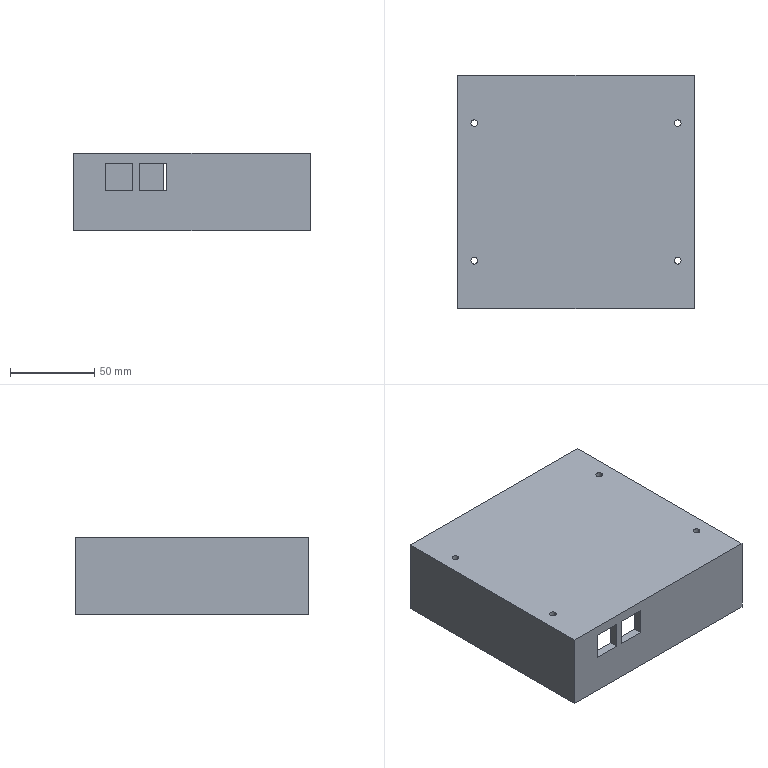Part | SolidWorks | features ICE 9, Extrusion 1, Shell 1 | 1 solid | 35 faces | box 140 x 138 x 46 mm | volume 201014 mm3 | plane 27 | cylinder 8 | commonest cylinder face diameters 4 x8
STEP:
#1=CARTESIAN_POINT('',(-39.512,8.412,41.));
#2=VERTEX_POINT('',#1);
#3=CARTESIAN_POINT('',(-35.512,8.412,41.));
#4=VERTEX_POINT('',#3);
#5=CARTESIAN_POINT('',(-37.512,8.412,41.));
#6=DIRECTION('',(0.,0.,1.));
#7=DIRECTION('',(1.,0.,0.));
#8=AXIS2_PLACEMENT_3D('',#5,#6,#7);
#9=CIRCLE('',#8,2.);
#10=EDGE_CURVE('',#2,#4,#9,.T.);
#11=ORIENTED_EDGE('',*,*,#10,.F.);
#12=CARTESIAN_POINT('',(-39.512,8.412,46.));
#13=VERTEX_POINT('',#12);
#14=CARTESIAN_POINT('',(-39.512,8.412,41.));
#15=DIRECTION('',(0.,0.,1.));
#16=VECTOR('',#15,1000.);
#17=LINE('',#14,#16);
#18=EDGE_CURVE('',#2,#13,#17,.T.);
#19=ORIENTED_EDGE('',*,*,#18,.T.);
#20=CARTESIAN_POINT('',(-35.512,8.412,46.));
#21=VERTEX_POINT('',#20);
#22=CARTESIAN_POINT('',(-37.512,8.412,46.));
#23=DIRECTION('',(0.,0.,1.));
#24=DIRECTION('',(1.,0.,0.));
#25=AXIS2_PLACEMENT_3D('',#22,#23,#24);
#26=CIRCLE('',#25,2.);
#27=EDGE_CURVE('',#13,#21,#26,.T.);
#28=ORIENTED_EDGE('',*,*,#27,.T.);
#29=CARTESIAN_POINT('',(-35.512,8.412,41.));
#30=DIRECTION('',(0.,0.,1.));
#31=VECTOR('',#30,1000.);
#32=LINE('',#29,#31);
#33=EDGE_CURVE('',#4,#21,#32,.T.);
#34=ORIENTED_EDGE('',*,*,#33,.F.);
#35=EDGE_LOOP('',(#11,#19,#28,#34));
#36=FACE_OUTER_BOUND('',#35,.T.);
#37=CARTESIAN_POINT('',(-37.512,8.412,41.));
#38=DIRECTION('',(0.,0.,1.));
#39=DIRECTION('',(1.,0.,0.));
#40=AXIS2_PLACEMENT_3D('',#37,#38,#39);
#41=CYLINDRICAL_SURFACE('',#40,2.);
#42=ADVANCED_FACE('',(#36),#41,.F.);
#43=CARTESIAN_POINT('',(80.888,89.812,41.));
#44=VERTEX_POINT('',#43);
#45=CARTESIAN_POINT('',(84.888,89.812,41.));
#46=VERTEX_POINT('',#45);
#47=CARTESIAN_POINT('',(82.888,89.812,41.));
#48=DIRECTION('',(0.,0.,1.));
#49=DIRECTION('',(1.,0.,0.));
#50=AXIS2_PLACEMENT_3D('',#47,#48,#49);
#51=CIRCLE('',#50,2.);
#52=EDGE_CURVE('',#44,#46,#51,.T.);
#53=ORIENTED_EDGE('',*,*,#52,.F.);
#54=CARTESIAN_POINT('',(80.888,89.812,46.));
#55=VERTEX_POINT('',#54);
#56=CARTESIAN_POINT('',(80.888,89.812,41.));
#57=DIRECTION('',(0.,0.,1.));
#58=VECTOR('',#57,1000.);
#59=LINE('',#56,#58);
#60=EDGE_CURVE('',#44,#55,#59,.T.);
#61=ORIENTED_EDGE('',*,*,#60,.T.);
#62=CARTESIAN_POINT('',(84.888,89.812,46.));
#63=VERTEX_POINT('',#62);
#64=CARTESIAN_POINT('',(82.888,89.812,46.));
#65=DIRECTION('',(0.,0.,1.));
#66=DIRECTION('',(1.,0.,0.));
#67=AXIS2_PLACEMENT_3D('',#64,#65,#66);
#68=CIRCLE('',#67,2.);
#69=EDGE_CURVE('',#55,#63,#68,.T.);
#70=ORIENTED_EDGE('',*,*,#69,.T.);
#71=CARTESIAN_POINT('',(84.888,89.812,41.));
#72=DIRECTION('',(0.,0.,1.));
#73=VECTOR('',#72,1000.);
#74=LINE('',#71,#73);
#75=EDGE_CURVE('',#46,#63,#74,.T.);
#76=ORIENTED_EDGE('',*,*,#75,.F.);
#77=EDGE_LOOP('',(#53,#61,#70,#76));
#78=FACE_OUTER_BOUND('',#77,.T.);
#79=CARTESIAN_POINT('',(82.888,89.812,41.));
#80=DIRECTION('',(0.,0.,1.));
#81=DIRECTION('',(1.,0.,0.));
#82=AXIS2_PLACEMENT_3D('',#79,#80,#81);
#83=CYLINDRICAL_SURFACE('',#82,2.);
#84=ADVANCED_FACE('',(#78),#83,.F.);
#85=CARTESIAN_POINT('',(80.888,8.412,41.));
#86=VERTEX_POINT('',#85);
#87=CARTESIAN_POINT('',(84.888,8.412,41.));
#88=VERTEX_POINT('',#87);
#89=CARTESIAN_POINT('',(82.888,8.412,41.));
#90=DIRECTION('',(0.,0.,1.));
#91=DIRECTION('',(1.,0.,0.));
#92=AXIS2_PLACEMENT_3D('',#89,#90,#91);
#93=CIRCLE('',#92,2.);
#94=EDGE_CURVE('',#86,#88,#93,.T.);
#95=ORIENTED_EDGE('',*,*,#94,.F.);
#96=CARTESIAN_POINT('',(80.888,8.412,46.));
#97=VERTEX_POINT('',#96);
#98=CARTESIAN_POINT('',(80.888,8.412,41.));
#99=DIRECTION('',(0.,0.,1.));
#100=VECTOR('',#99,1000.);
#101=LINE('',#98,#100);
#102=EDGE_CURVE('',#86,#97,#101,.T.);
#103=ORIENTED_EDGE('',*,*,#102,.T.);
#104=CARTESIAN_POINT('',(84.888,8.412,46.));
#105=VERTEX_POINT('',#104);
#106=CARTESIAN_POINT('',(82.888,8.412,46.));
#107=DIRECTION('',(0.,0.,1.));
#108=DIRECTION('',(1.,0.,0.));
#109=AXIS2_PLACEMENT_3D('',#106,#107,#108);
#110=CIRCLE('',#109,2.);
#111=EDGE_CURVE('',#97,#105,#110,.T.);
#112=ORIENTED_EDGE('',*,*,#111,.T.);
#113=CARTESIAN_POINT('',(84.888,8.412,41.));
#114=DIRECTION('',(0.,0.,1.));
#115=VECTOR('',#114,1000.);
#116=LINE('',#113,#115);
#117=EDGE_CURVE('',#88,#105,#116,.T.);
#118=ORIENTED_EDGE('',*,*,#117,.F.);
#119=EDGE_LOOP('',(#95,#103,#112,#118));
#120=FACE_OUTER_BOUND('',#119,.T.);
#121=CARTESIAN_POINT('',(82.888,8.412,41.));
#122=DIRECTION('',(0.,0.,1.));
#123=DIRECTION('',(1.,0.,0.));
#124=AXIS2_PLACEMENT_3D('',#121,#122,#123);
#125=CYLINDRICAL_SURFACE('',#124,2.);
#126=ADVANCED_FACE('',(#120),#125,.F.);
#127=CARTESIAN_POINT('',(-39.512,89.812,41.));
#128=VERTEX_POINT('',#127);
#129=CARTESIAN_POINT('',(-35.512,89.812,41.));
#130=VERTEX_POINT('',#129);
#131=CARTESIAN_POINT('',(-37.512,89.812,41.));
#132=DIRECTION('',(0.,0.,1.));
#133=DIRECTION('',(1.,0.,0.));
#134=AXIS2_PLACEMENT_3D('',#131,#132,#133);
#135=CIRCLE('',#134,2.);
#136=EDGE_CURVE('',#128,#130,#135,.T.);
#137=ORIENTED_EDGE('',*,*,#136,.F.);
#138=CARTESIAN_POINT('',(-39.512,89.812,46.));
#139=VERTEX_POINT('',#138);
#140=CARTESIAN_POINT('',(-39.512,89.812,41.));
#141=DIRECTION('',(0.,0.,1.));
#142=VECTOR('',#141,1000.);
#143=LINE('',#140,#142);
#144=EDGE_CURVE('',#128,#139,#143,.T.);
#145=ORIENTED_EDGE('',*,*,#144,.T.);
#146=CARTESIAN_POINT('',(-35.512,89.812,46.));
#147=VERTEX_POINT('',#146);
#148=CARTESIAN_POINT('',(-37.512,89.812,46.));
#149=DIRECTION('',(0.,0.,1.));
#150=DIRECTION('',(1.,0.,0.));
#151=AXIS2_PLACEMENT_3D('',#148,#149,#150);
#152=CIRCLE('',#151,2.);
#153=EDGE_CURVE('',#139,#147,#152,.T.);
#154=ORIENTED_EDGE('',*,*,#153,.T.);
#155=CARTESIAN_POINT('',(-35.512,89.812,41.));
#156=DIRECTION('',(0.,0.,1.));
#157=VECTOR('',#156,1000.);
#158=LINE('',#155,#157);
#159=EDGE_CURVE('',#130,#147,#158,.T.);
#160=ORIENTED_EDGE('',*,*,#159,.F.);
#161=EDGE_LOOP('',(#137,#145,#154,#160));
#162=FACE_OUTER_BOUND('',#161,.T.);
#163=CARTESIAN_POINT('',(-37.512,89.812,41.));
#164=DIRECTION('',(0.,0.,1.));
#165=DIRECTION('',(1.,0.,0.));
#166=AXIS2_PLACEMENT_3D('',#163,#164,#165);
#167=CYLINDRICAL_SURFACE('',#166,2.);
#168=ADVANCED_FACE('',(#162),#167,.F.);
#169=CARTESIAN_POINT('',(-47.312,118.112,0.));
#170=VERTEX_POINT('',#169);
#171=CARTESIAN_POINT('',(-47.312,-19.888,0.));
#172=VERTEX_POINT('',#171);
#173=CARTESIAN_POINT('',(-47.312,118.112,0.));
#174=DIRECTION('',(0.,-1.,0.));
#175=VECTOR('',#174,1000.);
#176=LINE('',#173,#175);
#177=EDGE_CURVE('',#170,#172,#176,.T.);
#178=ORIENTED_EDGE('',*,*,#177,.T.);
#179=CARTESIAN_POINT('',(-47.312,-19.888,46.));
#180=VERTEX_POINT('',#179);
#181=CARTESIAN_POINT('',(-47.312,-19.888,46.));
#182=DIRECTION('',(0.,0.,-1.));
#183=VECTOR('',#182,1000.);
#184=LINE('',#181,#183);
#185=EDGE_CURVE('',#180,#172,#184,.T.);
#186=ORIENTED_EDGE('',*,*,#185,.F.);
#187=CARTESIAN_POINT('',(-47.312,118.112,46.));
#188=VERTEX_POINT('',#187);
#189=CARTESIAN_POINT('',(-47.312,118.112,46.));
#190=DIRECTION('',(0.,-1.,0.));
#191=VECTOR('',#190,1000.);
#192=LINE('',#189,#191);
#193=EDGE_CURVE('',#188,#180,#192,.T.);
#194=ORIENTED_EDGE('',*,*,#193,.F.);
#195=CARTESIAN_POINT('',(-47.312,118.112,46.));
#196=DIRECTION('',(0.,0.,-1.));
#197=VECTOR('',#196,1000.);
#198=LINE('',#195,#197);
#199=EDGE_CURVE('',#188,#170,#198,.T.);
#200=ORIENTED_EDGE('',*,*,#199,.T.);
#201=EDGE_LOOP('',(#178,#186,#194,#200));
#202=FACE_OUTER_BOUND('',#201,.T.);
#203=CARTESIAN_POINT('',(-47.312,118.112,46.));
#204=DIRECTION('',(1.,0.,0.));
#205=DIRECTION('',(0.,1.,0.));
#206=AXIS2_PLACEMENT_3D('',#203,#204,#205);
#207=PLANE('',#206);
#208=ADVANCED_FACE('',(#202),#207,.F.);
#209=CARTESIAN_POINT('',(-8.312,-19.888,24.));
#210=VERTEX_POINT('',#209);
#211=CARTESIAN_POINT('',(7.688,-19.888,24.));
#212=VERTEX_POINT('',#211);
#213=CARTESIAN_POINT('',(-8.312,-19.888,24.));
#214=DIRECTION('',(1.,0.,0.));
#215=VECTOR('',#214,1000.);
#216=LINE('',#213,#215);
#217=EDGE_CURVE('',#210,#212,#216,.T.);
#218=ORIENTED_EDGE('',*,*,#217,.F.);
#219=CARTESIAN_POINT('',(-8.312,-19.888,40.));
#220=VERTEX_POINT('',#219);
#221=CARTESIAN_POINT('',(-8.312,-19.888,40.));
#222=DIRECTION('',(0.,0.,-1.));
#223=VECTOR('',#222,1000.);
#224=LINE('',#221,#223);
#225=EDGE_CURVE('',#220,#210,#224,.T.);
#226=ORIENTED_EDGE('',*,*,#225,.F.);
#227=CARTESIAN_POINT('',(7.688,-19.888,40.));
#228=VERTEX_POINT('',#227);
#229=CARTESIAN_POINT('',(-8.312,-19.888,40.));
#230=DIRECTION('',(-1.,0.,0.));
#231=VECTOR('',#230,1000.);
#232=LINE('',#229,#231);
#233=EDGE_CURVE('',#228,#220,#232,.T.);
#234=ORIENTED_EDGE('',*,*,#233,.F.);
#235=CARTESIAN_POINT('',(7.688,-19.888,40.));
#236=DIRECTION('',(0.,0.,1.));
#237=VECTOR('',#236,1000.);
#238=LINE('',#235,#237);
#239=EDGE_CURVE('',#212,#228,#238,.T.);
#240=ORIENTED_EDGE('',*,*,#239,.F.);
#241=EDGE_LOOP('',(#218,#226,#234,#240));
#242=FACE_BOUND('',#241,.T.);
#243=CARTESIAN_POINT('',(-28.312,-19.888,24.));
#244=VERTEX_POINT('',#243);
#245=CARTESIAN_POINT('',(-12.312,-19.888,24.));
#246=VERTEX_POINT('',#245);
#247=CARTESIAN_POINT('',(-28.312,-19.888,24.));
#248=DIRECTION('',(1.,0.,0.));
#249=VECTOR('',#248,1000.);
#250=LINE('',#247,#249);
#251=EDGE_CURVE('',#244,#246,#250,.T.);
#252=ORIENTED_EDGE('',*,*,#251,.F.);
#253=CARTESIAN_POINT('',(-28.312,-19.888,40.));
#254=VERTEX_POINT('',#253);
#255=CARTESIAN_POINT('',(-28.312,-19.888,40.));
#256=DIRECTION('',(0.,0.,-1.));
#257=VECTOR('',#256,1000.);
#258=LINE('',#255,#257);
#259=EDGE_CURVE('',#254,#244,#258,.T.);
#260=ORIENTED_EDGE('',*,*,#259,.F.);
#261=CARTESIAN_POINT('',(-12.312,-19.888,40.));
#262=VERTEX_POINT('',#261);
#263=CARTESIAN_POINT('',(-28.312,-19.888,40.));
#264=DIRECTION('',(-1.,0.,0.));
#265=VECTOR('',#264,1000.);
#266=LINE('',#263,#265);
#267=EDGE_CURVE('',#262,#254,#266,.T.);
#268=ORIENTED_EDGE('',*,*,#267,.F.);
#269=CARTESIAN_POINT('',(-12.312,-19.888,40.));
#270=DIRECTION('',(0.,0.,1.));
#271=VECTOR('',#270,1000.);
#272=LINE('',#269,#271);
#273=EDGE_CURVE('',#246,#262,#272,.T.);
#274=ORIENTED_EDGE('',*,*,#273,.F.);
#275=EDGE_LOOP('',(#252,#260,#268,#274));
#276=FACE_BOUND('',#275,.T.);
#277=CARTESIAN_POINT('',(92.688,-19.888,0.));
#278=VERTEX_POINT('',#277);
#279=CARTESIAN_POINT('',(-47.312,-19.888,0.));
#280=DIRECTION('',(1.,0.,0.));
#281=VECTOR('',#280,1000.);
#282=LINE('',#279,#281);
#283=EDGE_CURVE('',#172,#278,#282,.T.);
#284=ORIENTED_EDGE('',*,*,#283,.T.);
#285=CARTESIAN_POINT('',(92.688,-19.888,46.));
#286=VERTEX_POINT('',#285);
#287=CARTESIAN_POINT('',(92.688,-19.888,46.));
#288=DIRECTION('',(0.,0.,-1.));
#289=VECTOR('',#288,1000.);
#290=LINE('',#287,#289);
#291=EDGE_CURVE('',#286,#278,#290,.T.);
#292=ORIENTED_EDGE('',*,*,#291,.F.);
#293=CARTESIAN_POINT('',(-47.312,-19.888,46.));
#294=DIRECTION('',(1.,0.,0.));
#295=VECTOR('',#294,1000.);
#296=LINE('',#293,#295);
#297=EDGE_CURVE('',#180,#286,#296,.T.);
#298=ORIENTED_EDGE('',*,*,#297,.F.);
#299=ORIENTED_EDGE('',*,*,#185,.T.);
#300=EDGE_LOOP('',(#284,#292,#298,#299));
#301=FACE_OUTER_BOUND('',#300,.T.);
#302=CARTESIAN_POINT('',(-47.312,-19.888,46.));
#303=DIRECTION('',(0.,1.,0.));
#304=DIRECTION('',(0.,0.,1.));
#305=AXIS2_PLACEMENT_3D('',#302,#303,#304);
#306=PLANE('',#305);
#307=ADVANCED_FACE('',(#242,#276,#301),#306,.F.);
#308=CARTESIAN_POINT('',(92.688,118.112,0.));
#309=VERTEX_POINT('',#308);
#310=CARTESIAN_POINT('',(92.688,118.112,0.));
#311=DIRECTION('',(0.,1.,0.));
#312=VECTOR('',#311,1000.);
#313=LINE('',#310,#312);
#314=EDGE_CURVE('',#278,#309,#313,.T.);
#315=ORIENTED_EDGE('',*,*,#314,.T.);
#316=CARTESIAN_POINT('',(92.688,118.112,46.));
#317=VERTEX_POINT('',#316);
#318=CARTESIAN_POINT('',(92.688,118.112,46.));
#319=DIRECTION('',(0.,0.,-1.));
#320=VECTOR('',#319,1000.);
#321=LINE('',#318,#320);
#322=EDGE_CURVE('',#317,#309,#321,.T.);
#323=ORIENTED_EDGE('',*,*,#322,.F.);
#324=CARTESIAN_POINT('',(92.688,118.112,46.));
#325=DIRECTION('',(0.,1.,0.));
#326=VECTOR('',#325,1000.);
#327=LINE('',#324,#326);
#328=EDGE_CURVE('',#286,#317,#327,.T.);
#329=ORIENTED_EDGE('',*,*,#328,.F.);
#330=ORIENTED_EDGE('',*,*,#291,.T.);
#331=EDGE_LOOP('',(#315,#323,#329,#330));
#332=FACE_OUTER_BOUND('',#331,.T.);
#333=CARTESIAN_POINT('',(92.688,118.112,46.));
#334=DIRECTION('',(-1.,0.,0.));
#335=DIRECTION('',(0.,-1.,0.));
#336=AXIS2_PLACEMENT_3D('',#333,#334,#335);
#337=PLANE('',#336);
#338=ADVANCED_FACE('',(#332),#337,.F.);
#339=CARTESIAN_POINT('',(76.688,118.112,40.));
#340=VERTEX_POINT('',#339);
#341=CARTESIAN_POINT('',(76.688,118.112,25.));
#342=VERTEX_POINT('',#341);
#343=CARTESIAN_POINT('',(76.688,118.112,0.));
#344=DIRECTION('',(0.,0.,-1.));
#345=VECTOR('',#344,1000.);
#346=LINE('',#343,#345);
#347=EDGE_CURVE('',#340,#342,#346,.T.);
#348=ORIENTED_EDGE('',*,*,#347,.F.);
#349=CARTESIAN_POINT('',(61.688,118.112,40.));
#350=VERTEX_POINT('',#349);
#351=CARTESIAN_POINT('',(0.,118.112,40.));
#352=DIRECTION('',(1.,0.,0.));
#353=VECTOR('',#352,1000.);
#354=LINE('',#351,#353);
#355=EDGE_CURVE('',#350,#340,#354,.T.);
#356=ORIENTED_EDGE('',*,*,#355,.F.);
#357=CARTESIAN_POINT('',(61.688,118.112,25.));
#358=VERTEX_POINT('',#357);
#359=CARTESIAN_POINT('',(61.688,118.112,0.));
#360=DIRECTION('',(0.,0.,-1.));
#361=VECTOR('',#360,1000.);
#362=LINE('',#359,#361);
#363=EDGE_CURVE('',#350,#358,#362,.T.);
#364=ORIENTED_EDGE('',*,*,#363,.T.);
#365=CARTESIAN_POINT('',(0.,118.112,25.));
#366=DIRECTION('',(1.,0.,0.));
#367=VECTOR('',#366,1000.);
#368=LINE('',#365,#367);
#369=EDGE_CURVE('',#358,#342,#368,.T.);
#370=ORIENTED_EDGE('',*,*,#369,.T.);
#371=EDGE_LOOP('',(#348,#356,#364,#370));
#372=FACE_BOUND('',#371,.T.);
#373=CARTESIAN_POINT('',(22.688,118.112,40.));
#374=VERTEX_POINT('',#373);
#375=CARTESIAN_POINT('',(22.688,118.112,22.));
#376=VERTEX_POINT('',#375);
#377=CARTESIAN_POINT('',(22.688,118.112,0.));
#378=DIRECTION('',(0.,0.,-1.));
#379=VECTOR('',#378,1000.);
#380=LINE('',#377,#379);
#381=EDGE_CURVE('',#374,#376,#380,.T.);
#382=ORIENTED_EDGE('',*,*,#381,.F.);
#383=CARTESIAN_POINT('',(5.688,118.112,40.));
#384=VERTEX_POINT('',#383);
#385=CARTESIAN_POINT('',(0.,118.112,40.));
#386=DIRECTION('',(1.,0.,0.));
#387=VECTOR('',#386,1000.);
#388=LINE('',#385,#387);
#389=EDGE_CURVE('',#384,#374,#388,.T.);
#390=ORIENTED_EDGE('',*,*,#389,.F.);
#391=CARTESIAN_POINT('',(5.688,118.112,22.));
#392=VERTEX_POINT('',#391);
#393=CARTESIAN_POINT('',(5.688,118.112,0.));
#394=DIRECTION('',(0.,0.,-1.));
#395=VECTOR('',#394,1000.);
#396=LINE('',#393,#395);
#397=EDGE_CURVE('',#384,#392,#396,.T.);
#398=ORIENTED_EDGE('',*,*,#397,.T.);
#399=CARTESIAN_POINT('',(0.,118.112,22.));
#400=DIRECTION('',(1.,0.,0.));
#401=VECTOR('',#400,1000.);
#402=LINE('',#399,#401);
#403=EDGE_CURVE('',#392,#376,#402,.T.);
#404=ORIENTED_EDGE('',*,*,#403,.T.);
#405=EDGE_LOOP('',(#382,#390,#398,#404));
#406=FACE_BOUND('',#405,.T.);
#407=CARTESIAN_POINT('',(-47.312,118.112,0.));
#408=DIRECTION('',(-1.,0.,0.));
#409=VECTOR('',#408,1000.);
#410=LINE('',#407,#409);
#411=EDGE_CURVE('',#309,#170,#410,.T.);
#412=ORIENTED_EDGE('',*,*,#411,.T.);
#413=ORIENTED_EDGE('',*,*,#199,.F.);
#414=CARTESIAN_POINT('',(-47.312,118.112,46.));
#415=DIRECTION('',(-1.,0.,0.));
#416=VECTOR('',#415,1000.);
#417=LINE('',#414,#416);
#418=EDGE_CURVE('',#317,#188,#417,.T.);
#419=ORIENTED_EDGE('',*,*,#418,.F.);
#420=ORIENTED_EDGE('',*,*,#322,.T.);
#421=EDGE_LOOP('',(#412,#413,#419,#420));
#422=FACE_OUTER_BOUND('',#421,.T.);
#423=CARTESIAN_POINT('',(-47.312,118.112,46.));
#424=DIRECTION('',(0.,-1.,0.));
#425=DIRECTION('',(0.,0.,-1.));
#426=AXIS2_PLACEMENT_3D('',#423,#424,#425);
#427=PLANE('',#426);
#428=ADVANCED_FACE('',(#372,#406,#422),#427,.F.);
#429=CARTESIAN_POINT('',(-37.512,8.412,46.));
#430=DIRECTION('',(0.,0.,1.));
#431=DIRECTION('',(1.,0.,0.));
#432=AXIS2_PLACEMENT_3D('',#429,#430,#431);
#433=CIRCLE('',#432,2.);
#434=EDGE_CURVE('',#21,#13,#433,.T.);
#435=ORIENTED_EDGE('',*,*,#434,.F.);
#436=ORIENTED_EDGE('',*,*,#27,.F.);
#437=EDGE_LOOP('',(#435,#436));
#438=FACE_BOUND('',#437,.T.);
#439=CARTESIAN_POINT('',(82.888,89.812,46.));
#440=DIRECTION('',(0.,0.,1.));
#441=DIRECTION('',(1.,0.,0.));
#442=AXIS2_PLACEMENT_3D('',#439,#440,#441);
#443=CIRCLE('',#442,2.);
#444=EDGE_CURVE('',#63,#55,#443,.T.);
#445=ORIENTED_EDGE('',*,*,#444,.F.);
#446=ORIENTED_EDGE('',*,*,#69,.F.);
#447=EDGE_LOOP('',(#445,#446));
#448=FACE_BOUND('',#447,.T.);
#449=CARTESIAN_POINT('',(82.888,8.412,46.));
#450=DIRECTION('',(0.,0.,1.));
#451=DIRECTION('',(1.,0.,0.));
#452=AXIS2_PLACEMENT_3D('',#449,#450,#451);
#453=CIRCLE('',#452,2.);
#454=EDGE_CURVE('',#105,#97,#453,.T.);
#455=ORIENTED_EDGE('',*,*,#454,.F.);
#456=ORIENTED_EDGE('',*,*,#111,.F.);
#457=EDGE_LOOP('',(#455,#456));
#458=FACE_BOUND('',#457,.T.);
#459=CARTESIAN_POINT('',(-37.512,89.812,46.));
#460=DIRECTION('',(0.,0.,1.));
#461=DIRECTION('',(1.,0.,0.));
#462=AXIS2_PLACEMENT_3D('',#459,#460,#461);
#463=CIRCLE('',#462,2.);
#464=EDGE_CURVE('',#147,#139,#463,.T.);
#465=ORIENTED_EDGE('',*,*,#464,.F.);
#466=ORIENTED_EDGE('',*,*,#153,.F.);
#467=EDGE_LOOP('',(#465,#466));
#468=FACE_BOUND('',#467,.T.);
#469=ORIENTED_EDGE('',*,*,#193,.T.);
#470=ORIENTED_EDGE('',*,*,#297,.T.);
#471=ORIENTED_EDGE('',*,*,#328,.T.);
#472=ORIENTED_EDGE('',*,*,#418,.T.);
#473=EDGE_LOOP('',(#469,#470,#471,#472));
#474=FACE_OUTER_BOUND('',#473,.T.);
#475=CARTESIAN_POINT('',(0.,0.,46.));
#476=DIRECTION('',(0.,0.,1.));
#477=DIRECTION('',(1.,0.,0.));
#478=AXIS2_PLACEMENT_3D('',#475,#476,#477);
#479=PLANE('',#478);
#480=ADVANCED_FACE('',(#438,#448,#458,#468,#474),#479,.T.);
#481=CARTESIAN_POINT('',(87.688,113.112,0.));
#482=VERTEX_POINT('',#481);
#483=CARTESIAN_POINT('',(-42.312,113.112,0.));
#484=VERTEX_POINT('',#483);
#485=CARTESIAN_POINT('',(-47.312,113.112,0.));
#486=DIRECTION('',(-1.,0.,0.));
#487=VECTOR('',#486,1000.);
#488=LINE('',#485,#487);
#489=EDGE_CURVE('',#482,#484,#488,.T.);
#490=ORIENTED_EDGE('',*,*,#489,.T.);
#491=CARTESIAN_POINT('',(-42.312,-14.888,0.));
#492=VERTEX_POINT('',#491);
#493=CARTESIAN_POINT('',(-42.312,118.112,0.));
#494=DIRECTION('',(0.,-1.,0.));
#495=VECTOR('',#494,1000.);
#496=LINE('',#493,#495);
#497=EDGE_CURVE('',#484,#492,#496,.T.);
#498=ORIENTED_EDGE('',*,*,#497,.T.);
#499=CARTESIAN_POINT('',(87.688,-14.888,0.));
#500=VERTEX_POINT('',#499);
#501=CARTESIAN_POINT('',(-47.312,-14.888,0.));
#502=DIRECTION('',(1.,0.,0.));
#503=VECTOR('',#502,1000.);
#504=LINE('',#501,#503);
#505=EDGE_CURVE('',#492,#500,#504,.T.);
#506=ORIENTED_EDGE('',*,*,#505,.T.);
#507=CARTESIAN_POINT('',(87.688,118.112,0.));
#508=DIRECTION('',(0.,1.,0.));
#509=VECTOR('',#508,1000.);
#510=LINE('',#507,#509);
#511=EDGE_CURVE('',#500,#482,#510,.T.);
#512=ORIENTED_EDGE('',*,*,#511,.T.);
#513=EDGE_LOOP('',(#490,#498,#506,#512));
#514=FACE_BOUND('',#513,.T.);
#515=ORIENTED_EDGE('',*,*,#177,.F.);
#516=ORIENTED_EDGE('',*,*,#411,.F.);
#517=ORIENTED_EDGE('',*,*,#314,.F.);
#518=ORIENTED_EDGE('',*,*,#283,.F.);
#519=EDGE_LOOP('',(#515,#516,#517,#518));
#520=FACE_OUTER_BOUND('',#519,.T.);
#521=CARTESIAN_POINT('',(0.,0.,0.));
#522=DIRECTION('',(0.,0.,1.));
#523=DIRECTION('',(1.,0.,0.));
#524=AXIS2_PLACEMENT_3D('',#521,#522,#523);
#525=PLANE('',#524);
#526=ADVANCED_FACE('',(#514,#520),#525,.F.);
#527=ORIENTED_EDGE('',*,*,#497,.F.);
#528=CARTESIAN_POINT('',(-42.312,113.112,41.));
#529=VERTEX_POINT('',#528);
#530=CARTESIAN_POINT('',(-42.312,113.112,46.));
#531=DIRECTION('',(0.,0.,-1.));
#532=VECTOR('',#531,1000.);
#533=LINE('',#530,#532);
#534=EDGE_CURVE('',#529,#484,#533,.T.);
#535=ORIENTED_EDGE('',*,*,#534,.F.);
#536=CARTESIAN_POINT('',(-42.312,-14.888,41.));
#537=VERTEX_POINT('',#536);
#538=CARTESIAN_POINT('',(-42.312,118.112,41.));
#539=DIRECTION('',(0.,-1.,0.));
#540=VECTOR('',#539,1000.);
#541=LINE('',#538,#540);
#542=EDGE_CURVE('',#529,#537,#541,.T.);
#543=ORIENTED_EDGE('',*,*,#542,.T.);
#544=CARTESIAN_POINT('',(-42.312,-14.888,46.));
#545=DIRECTION('',(0.,0.,-1.));
#546=VECTOR('',#545,1000.);
#547=LINE('',#544,#546);
#548=EDGE_CURVE('',#537,#492,#547,.T.);
#549=ORIENTED_EDGE('',*,*,#548,.T.);
#550=EDGE_LOOP('',(#527,#535,#543,#549));
#551=FACE_OUTER_BOUND('',#550,.T.);
#552=CARTESIAN_POINT('',(-42.312,118.112,46.));
#553=DIRECTION('',(1.,0.,0.));
#554=DIRECTION('',(0.,1.,0.));
#555=AXIS2_PLACEMENT_3D('',#552,#553,#554);
#556=PLANE('',#555);
#557=ADVANCED_FACE('',(#551),#556,.T.);
#558=CARTESIAN_POINT('',(-8.312,-14.888,40.));
#559=VERTEX_POINT('',#558);
#560=CARTESIAN_POINT('',(-8.312,-14.888,24.));
#561=VERTEX_POINT('',#560);
#562=CARTESIAN_POINT('',(-8.312,-14.888,40.));
#563=DIRECTION('',(0.,0.,-1.));
#564=VECTOR('',#563,1000.);
#565=LINE('',#562,#564);
#566=EDGE_CURVE('',#559,#561,#565,.T.);
#567=ORIENTED_EDGE('',*,*,#566,.T.);
#568=CARTESIAN_POINT('',(7.688,-14.888,24.));
#569=VERTEX_POINT('',#568);
#570=CARTESIAN_POINT('',(-8.312,-14.888,24.));
#571=DIRECTION('',(1.,0.,0.));
#572=VECTOR('',#571,1000.);
#573=LINE('',#570,#572);
#574=EDGE_CURVE('',#561,#569,#573,.T.);
#575=ORIENTED_EDGE('',*,*,#574,.T.);
#576=CARTESIAN_POINT('',(7.688,-14.888,40.));
#577=VERTEX_POINT('',#576);
#578=CARTESIAN_POINT('',(7.688,-14.888,40.));
#579=DIRECTION('',(0.,0.,1.));
#580=VECTOR('',#579,1000.);
#581=LINE('',#578,#580);
#582=EDGE_CURVE('',#569,#577,#581,.T.);
#583=ORIENTED_EDGE('',*,*,#582,.T.);
#584=CARTESIAN_POINT('',(-8.312,-14.888,40.));
#585=DIRECTION('',(-1.,0.,0.));
#586=VECTOR('',#585,1000.);
#587=LINE('',#584,#586);
#588=EDGE_CURVE('',#577,#559,#587,.T.);
#589=ORIENTED_EDGE('',*,*,#588,.T.);
#590=EDGE_LOOP('',(#567,#575,#583,#589));
#591=FACE_BOUND('',#590,.T.);
#592=CARTESIAN_POINT('',(-28.312,-14.888,40.));
#593=VERTEX_POINT('',#592);
#594=CARTESIAN_POINT('',(-28.312,-14.888,24.));
#595=VERTEX_POINT('',#594);
#596=CARTESIAN_POINT('',(-28.312,-14.888,40.));
#597=DIRECTION('',(0.,0.,-1.));
#598=VECTOR('',#597,1000.);
#599=LINE('',#596,#598);
#600=EDGE_CURVE('',#593,#595,#599,.T.);
#601=ORIENTED_EDGE('',*,*,#600,.T.);
#602=CARTESIAN_POINT('',(-12.312,-14.888,24.));
#603=VERTEX_POINT('',#602);
#604=CARTESIAN_POINT('',(-28.312,-14.888,24.));
#605=DIRECTION('',(1.,0.,0.));
#606=VECTOR('',#605,1000.);
#607=LINE('',#604,#606);
#608=EDGE_CURVE('',#595,#603,#607,.T.);
#609=ORIENTED_EDGE('',*,*,#608,.T.);
#610=CARTESIAN_POINT('',(-12.312,-14.888,40.));
#611=VERTEX_POINT('',#610);
#612=CARTESIAN_POINT('',(-12.312,-14.888,40.));
#613=DIRECTION('',(0.,0.,1.));
#614=VECTOR('',#613,1000.);
#615=LINE('',#612,#614);
#616=EDGE_CURVE('',#603,#611,#615,.T.);
#617=ORIENTED_EDGE('',*,*,#616,.T.);
#618=CARTESIAN_POINT('',(-28.312,-14.888,40.));
#619=DIRECTION('',(-1.,0.,0.));
#620=VECTOR('',#619,1000.);
#621=LINE('',#618,#620);
#622=EDGE_CURVE('',#611,#593,#621,.T.);
#623=ORIENTED_EDGE('',*,*,#622,.T.);
#624=EDGE_LOOP('',(#601,#609,#617,#623));
#625=FACE_BOUND('',#624,.T.);
#626=ORIENTED_EDGE('',*,*,#505,.F.);
#627=ORIENTED_EDGE('',*,*,#548,.F.);
#628=CARTESIAN_POINT('',(87.688,-14.888,41.));
#629=VERTEX_POINT('',#628);
#630=CARTESIAN_POINT('',(-47.312,-14.888,41.));
#631=DIRECTION('',(1.,0.,0.));
#632=VECTOR('',#631,1000.);
#633=LINE('',#630,#632);
#634=EDGE_CURVE('',#537,#629,#633,.T.);
#635=ORIENTED_EDGE('',*,*,#634,.T.);
#636=CARTESIAN_POINT('',(87.688,-14.888,46.));
#637=DIRECTION('',(0.,0.,-1.));
#638=VECTOR('',#637,1000.);
#639=LINE('',#636,#638);
#640=EDGE_CURVE('',#629,#500,#639,.T.);
#641=ORIENTED_EDGE('',*,*,#640,.T.);
#642=EDGE_LOOP('',(#626,#627,#635,#641));
#643=FACE_OUTER_BOUND('',#642,.T.);
#644=CARTESIAN_POINT('',(-47.312,-14.888,46.));
#645=DIRECTION('',(0.,1.,0.));
#646=DIRECTION('',(0.,0.,1.));
#647=AXIS2_PLACEMENT_3D('',#644,#645,#646);
#648=PLANE('',#647);
#649=ADVANCED_FACE('',(#591,#625,#643),#648,.T.);
#650=ORIENTED_EDGE('',*,*,#511,.F.);
#651=ORIENTED_EDGE('',*,*,#640,.F.);
#652=CARTESIAN_POINT('',(87.688,113.112,41.));
#653=VERTEX_POINT('',#652);
#654=CARTESIAN_POINT('',(87.688,118.112,41.));
#655=DIRECTION('',(0.,1.,0.));
#656=VECTOR('',#655,1000.);
#657=LINE('',#654,#656);
#658=EDGE_CURVE('',#629,#653,#657,.T.);
#659=ORIENTED_EDGE('',*,*,#658,.T.);
#660=CARTESIAN_POINT('',(87.688,113.112,46.));
#661=DIRECTION('',(0.,0.,-1.));
#662=VECTOR('',#661,1000.);
#663=LINE('',#660,#662);
#664=EDGE_CURVE('',#653,#482,#663,.T.);
#665=ORIENTED_EDGE('',*,*,#664,.T.);
#666=EDGE_LOOP('',(#650,#651,#659,#665));
#667=FACE_OUTER_BOUND('',#666,.T.);
#668=CARTESIAN_POINT('',(87.688,118.112,46.));
#669=DIRECTION('',(-1.,0.,0.));
#670=DIRECTION('',(0.,-1.,0.));
#671=AXIS2_PLACEMENT_3D('',#668,#669,#670);
#672=PLANE('',#671);
#673=ADVANCED_FACE('',(#667),#672,.T.);
#674=CARTESIAN_POINT('',(61.688,113.112,40.));
#675=VERTEX_POINT('',#674);
#676=CARTESIAN_POINT('',(76.688,113.112,40.));
#677=VERTEX_POINT('',#676);
#678=CARTESIAN_POINT('',(0.,113.112,40.));
#679=DIRECTION('',(1.,0.,0.));
#680=VECTOR('',#679,1000.);
#681=LINE('',#678,#680);
#682=EDGE_CURVE('',#675,#677,#681,.T.);
#683=ORIENTED_EDGE('',*,*,#682,.T.);
#684=CARTESIAN_POINT('',(76.688,113.112,25.));
#685=VERTEX_POINT('',#684);
#686=CARTESIAN_POINT('',(76.688,113.112,0.));
#687=DIRECTION('',(0.,0.,-1.));
#688=VECTOR('',#687,1000.);
#689=LINE('',#686,#688);
#690=EDGE_CURVE('',#677,#685,#689,.T.);
#691=ORIENTED_EDGE('',*,*,#690,.T.);
#692=CARTESIAN_POINT('',(61.688,113.112,25.));
#693=VERTEX_POINT('',#692);
#694=CARTESIAN_POINT('',(0.,113.112,25.));
#695=DIRECTION('',(1.,0.,0.));
#696=VECTOR('',#695,1000.);
#697=LINE('',#694,#696);
#698=EDGE_CURVE('',#693,#685,#697,.T.);
#699=ORIENTED_EDGE('',*,*,#698,.F.);
#700=CARTESIAN_POINT('',(61.688,113.112,0.));
#701=DIRECTION('',(0.,0.,-1.));
#702=VECTOR('',#701,1000.);
#703=LINE('',#700,#702);
#704=EDGE_CURVE('',#675,#693,#703,.T.);
#705=ORIENTED_EDGE('',*,*,#704,.F.);
#706=EDGE_LOOP('',(#683,#691,#699,#705));
#707=FACE_BOUND('',#706,.T.);
#708=CARTESIAN_POINT('',(5.688,113.112,40.));
#709=VERTEX_POINT('',#708);
#710=CARTESIAN_POINT('',(22.688,113.112,40.));
#711=VERTEX_POINT('',#710);
#712=CARTESIAN_POINT('',(0.,113.112,40.));
#713=DIRECTION('',(1.,0.,0.));
#714=VECTOR('',#713,1000.);
#715=LINE('',#712,#714);
#716=EDGE_CURVE('',#709,#711,#715,.T.);
#717=ORIENTED_EDGE('',*,*,#716,.T.);
#718=CARTESIAN_POINT('',(22.688,113.112,22.));
#719=VERTEX_POINT('',#718);
#720=CARTESIAN_POINT('',(22.688,113.112,0.));
#721=DIRECTION('',(0.,0.,-1.));
#722=VECTOR('',#721,1000.);
#723=LINE('',#720,#722);
#724=EDGE_CURVE('',#711,#719,#723,.T.);
#725=ORIENTED_EDGE('',*,*,#724,.T.);
#726=CARTESIAN_POINT('',(5.688,113.112,22.));
#727=VERTEX_POINT('',#726);
#728=CARTESIAN_POINT('',(0.,113.112,22.));
#729=DIRECTION('',(1.,0.,0.));
#730=VECTOR('',#729,1000.);
#731=LINE('',#728,#730);
#732=EDGE_CURVE('',#727,#719,#731,.T.);
#733=ORIENTED_EDGE('',*,*,#732,.F.);
#734=CARTESIAN_POINT('',(5.688,113.112,0.));
#735=DIRECTION('',(0.,0.,-1.));
#736=VECTOR('',#735,1000.);
#737=LINE('',#734,#736);
#738=EDGE_CURVE('',#709,#727,#737,.T.);
#739=ORIENTED_EDGE('',*,*,#738,.F.);
#740=EDGE_LOOP('',(#717,#725,#733,#739));
#741=FACE_BOUND('',#740,.T.);
#742=ORIENTED_EDGE('',*,*,#489,.F.);
#743=ORIENTED_EDGE('',*,*,#664,.F.);
#744=CARTESIAN_POINT('',(-47.312,113.112,41.));
#745=DIRECTION('',(-1.,0.,0.));
#746=VECTOR('',#745,1000.);
#747=LINE('',#744,#746);
#748=EDGE_CURVE('',#653,#529,#747,.T.);
#749=ORIENTED_EDGE('',*,*,#748,.T.);
#750=ORIENTED_EDGE('',*,*,#534,.T.);
#751=EDGE_LOOP('',(#742,#743,#749,#750));
#752=FACE_OUTER_BOUND('',#751,.T.);
#753=CARTESIAN_POINT('',(-47.312,113.112,46.));
#754=DIRECTION('',(0.,-1.,0.));
#755=DIRECTION('',(0.,0.,-1.));
#756=AXIS2_PLACEMENT_3D('',#753,#754,#755);
#757=PLANE('',#756);
#758=ADVANCED_FACE('',(#707,#741,#752),#757,.T.);
#759=CARTESIAN_POINT('',(-37.512,8.412,41.));
#760=DIRECTION('',(0.,0.,1.));
#761=DIRECTION('',(1.,0.,0.));
#762=AXIS2_PLACEMENT_3D('',#759,#760,#761);
#763=CIRCLE('',#762,2.);
#764=EDGE_CURVE('',#4,#2,#763,.T.);
#765=ORIENTED_EDGE('',*,*,#764,.T.);
#766=ORIENTED_EDGE('',*,*,#10,.T.);
#767=EDGE_LOOP('',(#765,#766));
#768=FACE_BOUND('',#767,.T.);
#769=CARTESIAN_POINT('',(82.888,89.812,41.));
#770=DIRECTION('',(0.,0.,1.));
#771=DIRECTION('',(1.,0.,0.));
#772=AXIS2_PLACEMENT_3D('',#769,#770,#771);
#773=CIRCLE('',#772,2.);
#774=EDGE_CURVE('',#46,#44,#773,.T.);
#775=ORIENTED_EDGE('',*,*,#774,.T.);
#776=ORIENTED_EDGE('',*,*,#52,.T.);
#777=EDGE_LOOP('',(#775,#776));
#778=FACE_BOUND('',#777,.T.);
#779=CARTESIAN_POINT('',(82.888,8.412,41.));
#780=DIRECTION('',(0.,0.,1.));
#781=DIRECTION('',(1.,0.,0.));
#782=AXIS2_PLACEMENT_3D('',#779,#780,#781);
#783=CIRCLE('',#782,2.);
#784=EDGE_CURVE('',#88,#86,#783,.T.);
#785=ORIENTED_EDGE('',*,*,#784,.T.);
#786=ORIENTED_EDGE('',*,*,#94,.T.);
#787=EDGE_LOOP('',(#785,#786));
#788=FACE_BOUND('',#787,.T.);
#789=CARTESIAN_POINT('',(-37.512,89.812,41.));
#790=DIRECTION('',(0.,0.,1.));
#791=DIRECTION('',(1.,0.,0.));
#792=AXIS2_PLACEMENT_3D('',#789,#790,#791);
#793=CIRCLE('',#792,2.);
#794=EDGE_CURVE('',#130,#128,#793,.T.);
#795=ORIENTED_EDGE('',*,*,#794,.T.);
#796=ORIENTED_EDGE('',*,*,#136,.T.);
#797=EDGE_LOOP('',(#795,#796));
#798=FACE_BOUND('',#797,.T.);
#799=ORIENTED_EDGE('',*,*,#542,.F.);
#800=ORIENTED_EDGE('',*,*,#748,.F.);
#801=ORIENTED_EDGE('',*,*,#658,.F.);
#802=ORIENTED_EDGE('',*,*,#634,.F.);
#803=EDGE_LOOP('',(#799,#800,#801,#802));
#804=FACE_OUTER_BOUND('',#803,.T.);
#805=CARTESIAN_POINT('',(0.,0.,41.));
#806=DIRECTION('',(0.,0.,1.));
#807=DIRECTION('',(1.,0.,0.));
#808=AXIS2_PLACEMENT_3D('',#805,#806,#807);
#809=PLANE('',#808);
#810=ADVANCED_FACE('',(#768,#778,#788,#798,#804),#809,.F.);
#811=ORIENTED_EDGE('',*,*,#389,.T.);
#812=CARTESIAN_POINT('',(22.688,113.112,40.));
#813=DIRECTION('',(0.,1.,0.));
#814=VECTOR('',#813,1000.);
#815=LINE('',#812,#814);
#816=EDGE_CURVE('',#711,#374,#815,.T.);
#817=ORIENTED_EDGE('',*,*,#816,.F.);
#818=ORIENTED_EDGE('',*,*,#716,.F.);
#819=CARTESIAN_POINT('',(5.688,113.112,40.));
#820=DIRECTION('',(0.,1.,0.));
#821=VECTOR('',#820,1000.);
#822=LINE('',#819,#821);
#823=EDGE_CURVE('',#709,#384,#822,.T.);
#824=ORIENTED_EDGE('',*,*,#823,.T.);
#825=EDGE_LOOP('',(#811,#817,#818,#824));
#826=FACE_OUTER_BOUND('',#825,.T.);
#827=CARTESIAN_POINT('',(0.,113.112,40.));
#828=DIRECTION('',(0.,0.,1.));
#829=DIRECTION('',(1.,0.,0.));
#830=AXIS2_PLACEMENT_3D('',#827,#828,#829);
#831=PLANE('',#830);
#832=ADVANCED_FACE('',(#826),#831,.F.);
#833=ORIENTED_EDGE('',*,*,#397,.F.);
#834=ORIENTED_EDGE('',*,*,#823,.F.);
#835=ORIENTED_EDGE('',*,*,#738,.T.);
#836=CARTESIAN_POINT('',(5.688,113.112,22.));
#837=DIRECTION('',(0.,1.,0.));
#838=VECTOR('',#837,1000.);
#839=LINE('',#836,#838);
#840=EDGE_CURVE('',#727,#392,#839,.T.);
#841=ORIENTED_EDGE('',*,*,#840,.T.);
#842=EDGE_LOOP('',(#833,#834,#835,#841));
#843=FACE_OUTER_BOUND('',#842,.T.);
#844=CARTESIAN_POINT('',(5.688,113.112,0.));
#845=DIRECTION('',(1.,0.,0.));
#846=DIRECTION('',(0.,0.,-1.));
#847=AXIS2_PLACEMENT_3D('',#844,#845,#846);
#848=PLANE('',#847);
#849=ADVANCED_FACE('',(#843),#848,.T.);
#850=ORIENTED_EDGE('',*,*,#403,.F.);
#851=ORIENTED_EDGE('',*,*,#840,.F.);
#852=ORIENTED_EDGE('',*,*,#732,.T.);
#853=CARTESIAN_POINT('',(22.688,113.112,22.));
#854=DIRECTION('',(0.,1.,0.));
#855=VECTOR('',#854,1000.);
#856=LINE('',#853,#855);
#857=EDGE_CURVE('',#719,#376,#856,.T.);
#858=ORIENTED_EDGE('',*,*,#857,.T.);
#859=EDGE_LOOP('',(#850,#851,#852,#858));
#860=FACE_OUTER_BOUND('',#859,.T.);
#861=CARTESIAN_POINT('',(0.,113.112,22.));
#862=DIRECTION('',(0.,0.,1.));
#863=DIRECTION('',(1.,0.,0.));
#864=AXIS2_PLACEMENT_3D('',#861,#862,#863);
#865=PLANE('',#864);
#866=ADVANCED_FACE('',(#860),#865,.T.);
#867=ORIENTED_EDGE('',*,*,#381,.T.);
#868=ORIENTED_EDGE('',*,*,#857,.F.);
#869=ORIENTED_EDGE('',*,*,#724,.F.);
#870=ORIENTED_EDGE('',*,*,#816,.T.);
#871=EDGE_LOOP('',(#867,#868,#869,#870));
#872=FACE_OUTER_BOUND('',#871,.T.);
#873=CARTESIAN_POINT('',(22.688,113.112,0.));
#874=DIRECTION('',(1.,0.,0.));
#875=DIRECTION('',(0.,0.,-1.));
#876=AXIS2_PLACEMENT_3D('',#873,#874,#875);
#877=PLANE('',#876);
#878=ADVANCED_FACE('',(#872),#877,.F.);
#879=ORIENTED_EDGE('',*,*,#355,.T.);
#880=CARTESIAN_POINT('',(76.688,113.112,40.));
#881=DIRECTION('',(0.,1.,0.));
#882=VECTOR('',#881,1000.);
#883=LINE('',#880,#882);
#884=EDGE_CURVE('',#677,#340,#883,.T.);
#885=ORIENTED_EDGE('',*,*,#884,.F.);
#886=ORIENTED_EDGE('',*,*,#682,.F.);
#887=CARTESIAN_POINT('',(61.688,113.112,40.));
#888=DIRECTION('',(0.,1.,0.));
#889=VECTOR('',#888,1000.);
#890=LINE('',#887,#889);
#891=EDGE_CURVE('',#675,#350,#890,.T.);
#892=ORIENTED_EDGE('',*,*,#891,.T.);
#893=EDGE_LOOP('',(#879,#885,#886,#892));
#894=FACE_OUTER_BOUND('',#893,.T.);
#895=CARTESIAN_POINT('',(0.,113.112,40.));
#896=DIRECTION('',(0.,0.,1.));
#897=DIRECTION('',(1.,0.,0.));
#898=AXIS2_PLACEMENT_3D('',#895,#896,#897);
#899=PLANE('',#898);
#900=ADVANCED_FACE('',(#894),#899,.F.);
#901=ORIENTED_EDGE('',*,*,#363,.F.);
#902=ORIENTED_EDGE('',*,*,#891,.F.);
#903=ORIENTED_EDGE('',*,*,#704,.T.);
#904=CARTESIAN_POINT('',(61.688,113.112,25.));
#905=DIRECTION('',(0.,1.,0.));
#906=VECTOR('',#905,1000.);
#907=LINE('',#904,#906);
#908=EDGE_CURVE('',#693,#358,#907,.T.);
#909=ORIENTED_EDGE('',*,*,#908,.T.);
#910=EDGE_LOOP('',(#901,#902,#903,#909));
#911=FACE_OUTER_BOUND('',#910,.T.);
#912=CARTESIAN_POINT('',(61.688,113.112,0.));
#913=DIRECTION('',(1.,0.,0.));
#914=DIRECTION('',(0.,0.,-1.));
#915=AXIS2_PLACEMENT_3D('',#912,#913,#914);
#916=PLANE('',#915);
#917=ADVANCED_FACE('',(#911),#916,.T.);
#918=ORIENTED_EDGE('',*,*,#369,.F.);
#919=ORIENTED_EDGE('',*,*,#908,.F.);
#920=ORIENTED_EDGE('',*,*,#698,.T.);
#921=CARTESIAN_POINT('',(76.688,113.112,25.));
#922=DIRECTION('',(0.,1.,0.));
#923=VECTOR('',#922,1000.);
#924=LINE('',#921,#923);
#925=EDGE_CURVE('',#685,#342,#924,.T.);
#926=ORIENTED_EDGE('',*,*,#925,.T.);
#927=EDGE_LOOP('',(#918,#919,#920,#926));
#928=FACE_OUTER_BOUND('',#927,.T.);
#929=CARTESIAN_POINT('',(0.,113.112,25.));
#930=DIRECTION('',(0.,0.,1.));
#931=DIRECTION('',(1.,0.,0.));
#932=AXIS2_PLACEMENT_3D('',#929,#930,#931);
#933=PLANE('',#932);
#934=ADVANCED_FACE('',(#928),#933,.T.);
#935=ORIENTED_EDGE('',*,*,#347,.T.);
#936=ORIENTED_EDGE('',*,*,#925,.F.);
#937=ORIENTED_EDGE('',*,*,#690,.F.);
#938=ORIENTED_EDGE('',*,*,#884,.T.);
#939=EDGE_LOOP('',(#935,#936,#937,#938));
#940=FACE_OUTER_BOUND('',#939,.T.);
#941=CARTESIAN_POINT('',(76.688,113.112,0.));
#942=DIRECTION('',(1.,0.,0.));
#943=DIRECTION('',(0.,0.,-1.));
#944=AXIS2_PLACEMENT_3D('',#941,#942,#943);
#945=PLANE('',#944);
#946=ADVANCED_FACE('',(#940),#945,.F.);
#947=ORIENTED_EDGE('',*,*,#144,.F.);
#948=ORIENTED_EDGE('',*,*,#794,.F.);
#949=ORIENTED_EDGE('',*,*,#159,.T.);
#950=ORIENTED_EDGE('',*,*,#464,.T.);
#951=EDGE_LOOP('',(#947,#948,#949,#950));
#952=FACE_OUTER_BOUND('',#951,.T.);
#953=CARTESIAN_POINT('',(-37.512,89.812,41.));
#954=DIRECTION('',(0.,0.,1.));
#955=DIRECTION('',(1.,0.,0.));
#956=AXIS2_PLACEMENT_3D('',#953,#954,#955);
#957=CYLINDRICAL_SURFACE('',#956,2.);
#958=ADVANCED_FACE('',(#952),#957,.F.);
#959=ORIENTED_EDGE('',*,*,#102,.F.);
#960=ORIENTED_EDGE('',*,*,#784,.F.);
#961=ORIENTED_EDGE('',*,*,#117,.T.);
#962=ORIENTED_EDGE('',*,*,#454,.T.);
#963=EDGE_LOOP('',(#959,#960,#961,#962));
#964=FACE_OUTER_BOUND('',#963,.T.);
#965=CARTESIAN_POINT('',(82.888,8.412,41.));
#966=DIRECTION('',(0.,0.,1.));
#967=DIRECTION('',(1.,0.,0.));
#968=AXIS2_PLACEMENT_3D('',#965,#966,#967);
#969=CYLINDRICAL_SURFACE('',#968,2.);
#970=ADVANCED_FACE('',(#964),#969,.F.);
#971=ORIENTED_EDGE('',*,*,#60,.F.);
#972=ORIENTED_EDGE('',*,*,#774,.F.);
#973=ORIENTED_EDGE('',*,*,#75,.T.);
#974=ORIENTED_EDGE('',*,*,#444,.T.);
#975=EDGE_LOOP('',(#971,#972,#973,#974));
#976=FACE_OUTER_BOUND('',#975,.T.);
#977=CARTESIAN_POINT('',(82.888,89.812,41.));
#978=DIRECTION('',(0.,0.,1.));
#979=DIRECTION('',(1.,0.,0.));
#980=AXIS2_PLACEMENT_3D('',#977,#978,#979);
#981=CYLINDRICAL_SURFACE('',#980,2.);
#982=ADVANCED_FACE('',(#976),#981,.F.);
#983=ORIENTED_EDGE('',*,*,#18,.F.);
#984=ORIENTED_EDGE('',*,*,#764,.F.);
#985=ORIENTED_EDGE('',*,*,#33,.T.);
#986=ORIENTED_EDGE('',*,*,#434,.T.);
#987=EDGE_LOOP('',(#983,#984,#985,#986));
#988=FACE_OUTER_BOUND('',#987,.T.);
#989=CARTESIAN_POINT('',(-37.512,8.412,41.));
#990=DIRECTION('',(0.,0.,1.));
#991=DIRECTION('',(1.,0.,0.));
#992=AXIS2_PLACEMENT_3D('',#989,#990,#991);
#993=CYLINDRICAL_SURFACE('',#992,2.);
#994=ADVANCED_FACE('',(#988),#993,.F.);
#995=ORIENTED_EDGE('',*,*,#259,.T.);
#996=CARTESIAN_POINT('',(-28.312,-14.888,24.));
#997=DIRECTION('',(0.,-1.,0.));
#998=VECTOR('',#997,1000.);
#999=LINE('',#996,#998);
#1000=EDGE_CURVE('',#595,#244,#999,.T.);
#1001=ORIENTED_EDGE('',*,*,#1000,.F.);
#1002=ORIENTED_EDGE('',*,*,#600,.F.);
#1003=CARTESIAN_POINT('',(-28.312,-14.888,40.));
#1004=DIRECTION('',(0.,-1.,0.));
#1005=VECTOR('',#1004,1000.);
#1006=LINE('',#1003,#1005);
#1007=EDGE_CURVE('',#593,#254,#1006,.T.);
#1008=ORIENTED_EDGE('',*,*,#1007,.T.);
#1009=EDGE_LOOP('',(#995,#1001,#1002,#1008));
#1010=FACE_OUTER_BOUND('',#1009,.T.);
#1011=CARTESIAN_POINT('',(-28.312,-14.888,40.));
#1012=DIRECTION('',(-1.,0.,0.));
#1013=DIRECTION('',(0.,0.,1.));
#1014=AXIS2_PLACEMENT_3D('',#1011,#1012,#1013);
#1015=PLANE('',#1014);
#1016=ADVANCED_FACE('',(#1010),#1015,.F.);
#1017=ORIENTED_EDGE('',*,*,#267,.T.);
#1018=ORIENTED_EDGE('',*,*,#1007,.F.);
#1019=ORIENTED_EDGE('',*,*,#622,.F.);
#1020=CARTESIAN_POINT('',(-12.312,-14.888,40.));
#1021=DIRECTION('',(0.,-1.,0.));
#1022=VECTOR('',#1021,1000.);
#1023=LINE('',#1020,#1022);
#1024=EDGE_CURVE('',#611,#262,#1023,.T.);
#1025=ORIENTED_EDGE('',*,*,#1024,.T.);
#1026=EDGE_LOOP('',(#1017,#1018,#1019,#1025));
#1027=FACE_OUTER_BOUND('',#1026,.T.);
#1028=CARTESIAN_POINT('',(-28.312,-14.888,40.));
#1029=DIRECTION('',(0.,0.,1.));
#1030=DIRECTION('',(1.,0.,0.));
#1031=AXIS2_PLACEMENT_3D('',#1028,#1029,#1030);
#1032=PLANE('',#1031);
#1033=ADVANCED_FACE('',(#1027),#1032,.F.);
#1034=ORIENTED_EDGE('',*,*,#273,.T.);
#1035=ORIENTED_EDGE('',*,*,#1024,.F.);
#1036=ORIENTED_EDGE('',*,*,#616,.F.);
#1037=CARTESIAN_POINT('',(-12.312,-14.888,24.));
#1038=DIRECTION('',(0.,-1.,0.));
#1039=VECTOR('',#1038,1000.);
#1040=LINE('',#1037,#1039);
#1041=EDGE_CURVE('',#603,#246,#1040,.T.);
#1042=ORIENTED_EDGE('',*,*,#1041,.T.);
#1043=EDGE_LOOP('',(#1034,#1035,#1036,#1042));
#1044=FACE_OUTER_BOUND('',#1043,.T.);
#1045=CARTESIAN_POINT('',(-12.312,-14.888,40.));
#1046=DIRECTION('',(1.,0.,0.));
#1047=DIRECTION('',(0.,0.,-1.));
#1048=AXIS2_PLACEMENT_3D('',#1045,#1046,#1047);
#1049=PLANE('',#1048);
#1050=ADVANCED_FACE('',(#1044),#1049,.F.);
#1051=ORIENTED_EDGE('',*,*,#251,.T.);
#1052=ORIENTED_EDGE('',*,*,#1041,.F.);
#1053=ORIENTED_EDGE('',*,*,#608,.F.);
#1054=ORIENTED_EDGE('',*,*,#1000,.T.);
#1055=EDGE_LOOP('',(#1051,#1052,#1053,#1054));
#1056=FACE_OUTER_BOUND('',#1055,.T.);
#1057=CARTESIAN_POINT('',(-28.312,-14.888,24.));
#1058=DIRECTION('',(0.,0.,-1.));
#1059=DIRECTION('',(-1.,0.,0.));
#1060=AXIS2_PLACEMENT_3D('',#1057,#1058,#1059);
#1061=PLANE('',#1060);
#1062=ADVANCED_FACE('',(#1056),#1061,.F.);
#1063=ORIENTED_EDGE('',*,*,#225,.T.);
#1064=CARTESIAN_POINT('',(-8.312,-14.888,24.));
#1065=DIRECTION('',(0.,-1.,0.));
#1066=VECTOR('',#1065,1000.);
#1067=LINE('',#1064,#1066);
#1068=EDGE_CURVE('',#561,#210,#1067,.T.);
#1069=ORIENTED_EDGE('',*,*,#1068,.F.);
#1070=ORIENTED_EDGE('',*,*,#566,.F.);
#1071=CARTESIAN_POINT('',(-8.312,-14.888,40.));
#1072=DIRECTION('',(0.,-1.,0.));
#1073=VECTOR('',#1072,1000.);
#1074=LINE('',#1071,#1073);
#1075=EDGE_CURVE('',#559,#220,#1074,.T.);
#1076=ORIENTED_EDGE('',*,*,#1075,.T.);
#1077=EDGE_LOOP('',(#1063,#1069,#1070,#1076));
#1078=FACE_OUTER_BOUND('',#1077,.T.);
#1079=CARTESIAN_POINT('',(-8.312,-14.888,40.));
#1080=DIRECTION('',(-1.,0.,0.));
#1081=DIRECTION('',(0.,0.,1.));
#1082=AXIS2_PLACEMENT_3D('',#1079,#1080,#1081);
#1083=PLANE('',#1082);
#1084=ADVANCED_FACE('',(#1078),#1083,.F.);
#1085=ORIENTED_EDGE('',*,*,#233,.T.);
#1086=ORIENTED_EDGE('',*,*,#1075,.F.);
#1087=ORIENTED_EDGE('',*,*,#588,.F.);
#1088=CARTESIAN_POINT('',(7.688,-14.888,40.));
#1089=DIRECTION('',(0.,-1.,0.));
#1090=VECTOR('',#1089,1000.);
#1091=LINE('',#1088,#1090);
#1092=EDGE_CURVE('',#577,#228,#1091,.T.);
#1093=ORIENTED_EDGE('',*,*,#1092,.T.);
#1094=EDGE_LOOP('',(#1085,#1086,#1087,#1093));
#1095=FACE_OUTER_BOUND('',#1094,.T.);
#1096=CARTESIAN_POINT('',(-8.312,-14.888,40.));
#1097=DIRECTION('',(0.,0.,1.));
#1098=DIRECTION('',(1.,0.,0.));
#1099=AXIS2_PLACEMENT_3D('',#1096,#1097,#1098);
#1100=PLANE('',#1099);
#1101=ADVANCED_FACE('',(#1095),#1100,.F.);
#1102=ORIENTED_EDGE('',*,*,#239,.T.);
#1103=ORIENTED_EDGE('',*,*,#1092,.F.);
#1104=ORIENTED_EDGE('',*,*,#582,.F.);
#1105=CARTESIAN_POINT('',(7.688,-14.888,24.));
#1106=DIRECTION('',(0.,-1.,0.));
#1107=VECTOR('',#1106,1000.);
#1108=LINE('',#1105,#1107);
#1109=EDGE_CURVE('',#569,#212,#1108,.T.);
#1110=ORIENTED_EDGE('',*,*,#1109,.T.);
#1111=EDGE_LOOP('',(#1102,#1103,#1104,#1110));
#1112=FACE_OUTER_BOUND('',#1111,.T.);
#1113=CARTESIAN_POINT('',(7.688,-14.888,40.));
#1114=DIRECTION('',(1.,0.,0.));
#1115=DIRECTION('',(0.,0.,-1.));
#1116=AXIS2_PLACEMENT_3D('',#1113,#1114,#1115);
#1117=PLANE('',#1116);
#1118=ADVANCED_FACE('',(#1112),#1117,.F.);
#1119=ORIENTED_EDGE('',*,*,#217,.T.);
#1120=ORIENTED_EDGE('',*,*,#1109,.F.);
#1121=ORIENTED_EDGE('',*,*,#574,.F.);
#1122=ORIENTED_EDGE('',*,*,#1068,.T.);
#1123=EDGE_LOOP('',(#1119,#1120,#1121,#1122));
#1124=FACE_OUTER_BOUND('',#1123,.T.);
#1125=CARTESIAN_POINT('',(-8.312,-14.888,24.));
#1126=DIRECTION('',(0.,0.,-1.));
#1127=DIRECTION('',(-1.,0.,0.));
#1128=AXIS2_PLACEMENT_3D('',#1125,#1126,#1127);
#1129=PLANE('',#1128);
#1130=ADVANCED_FACE('',(#1124),#1129,.F.);
#1131=CLOSED_SHELL('',(#42,#84,#126,#168,#208,#307,#338,#428,#480,#526,#557,#649,#673,#758,#810,#832,#849,#866,#878,#900,#917,#934,#946,#958,#970,#982,#994,#1016,#1033,#1050,#1062,#1084,#1101,#1118,#1130));
#1132=MANIFOLD_SOLID_BREP('',#1131);
#1133=CARTESIAN_POINT('',(0.,0.,0.));
#1134=DIRECTION('',(0.,0.,1.));
#1135=DIRECTION('',(1.,0.,0.));
#1136=AXIS2_PLACEMENT_3D('',#1133,#1134,#1135);
#1137=(LENGTH_UNIT()NAMED_UNIT(*)SI_UNIT(.MILLI.,.METRE.));
#1138=UNCERTAINTY_MEASURE_WITH_UNIT(LENGTH_MEASURE(0.00001),#1137,'','');
#1139=(NAMED_UNIT(*)PLANE_ANGLE_UNIT()SI_UNIT($,.RADIAN.));
#1140=(NAMED_UNIT(*)SI_UNIT($,.STERADIAN.)SOLID_ANGLE_UNIT());
#1141=(GEOMETRIC_REPRESENTATION_CONTEXT(3)GLOBAL_UNCERTAINTY_ASSIGNED_CONTEXT((#1138))GLOBAL_UNIT_ASSIGNED_CONTEXT((#1137,#1139,#1140))REPRESENTATION_CONTEXT('',''));
#1142=ADVANCED_BREP_SHAPE_REPRESENTATION('',(#1132,#1136),#1141);